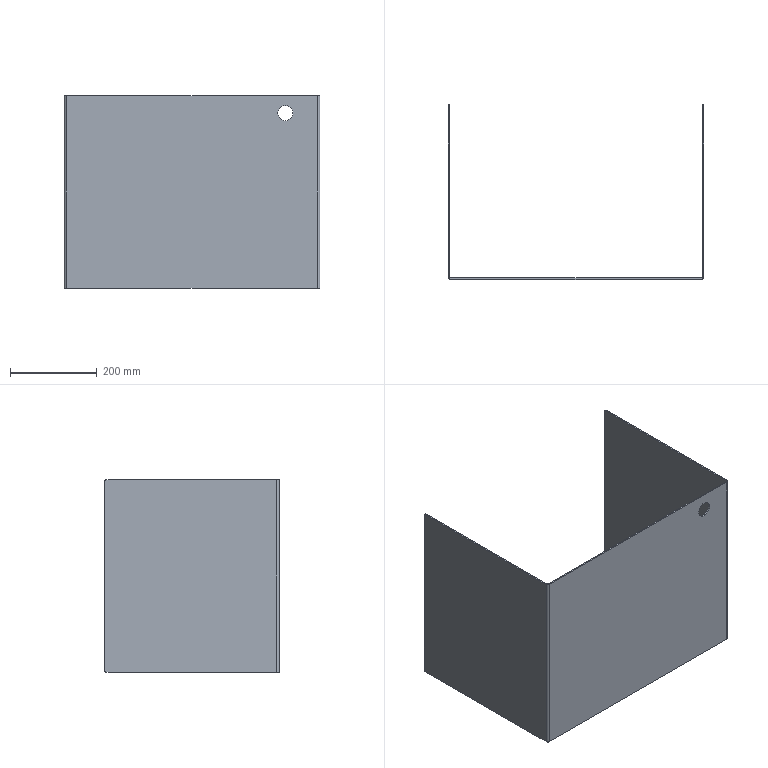Part | SolidWorks | features Fillet 1, FlatPattern 1, ICE 1, SMBaseFlange 1, SheetMetal 1 | 1 solid | 28 faces | box 590 x 403 x 444 mm | volume 1843422 mm3 | plane 18 | cylinder 10 | commonest cylinder face diameters 6.4 x4 6 x2 12 x2 35 x2
STEP:
#1=CARTESIAN_POINT('',(510.,0.,164.5));
#2=VERTEX_POINT('',#1);
#3=CARTESIAN_POINT('',(510.,0.,199.5));
#4=VERTEX_POINT('',#3);
#5=CARTESIAN_POINT('',(510.,0.,182.));
#6=DIRECTION('',(0.,1.,0.));
#7=DIRECTION('',(0.,0.,1.));
#8=AXIS2_PLACEMENT_3D('',#5,#6,#7);
#9=CIRCLE('',#8,17.5);
#10=EDGE_CURVE('',#2,#4,#9,.T.);
#11=ORIENTED_EDGE('',*,*,#10,.F.);
#12=CARTESIAN_POINT('',(510.,3.,164.5));
#13=VERTEX_POINT('',#12);
#14=CARTESIAN_POINT('',(510.,0.,164.5));
#15=DIRECTION('',(0.,1.,0.));
#16=VECTOR('',#15,1000.);
#17=LINE('',#14,#16);
#18=EDGE_CURVE('',#2,#13,#17,.T.);
#19=ORIENTED_EDGE('',*,*,#18,.T.);
#20=CARTESIAN_POINT('',(510.,3.,199.5));
#21=VERTEX_POINT('',#20);
#22=CARTESIAN_POINT('',(510.,3.,182.));
#23=DIRECTION('',(0.,1.,0.));
#24=DIRECTION('',(0.,0.,1.));
#25=AXIS2_PLACEMENT_3D('',#22,#23,#24);
#26=CIRCLE('',#25,17.5);
#27=EDGE_CURVE('',#13,#21,#26,.T.);
#28=ORIENTED_EDGE('',*,*,#27,.T.);
#29=CARTESIAN_POINT('',(510.,0.,199.5));
#30=DIRECTION('',(0.,1.,0.));
#31=VECTOR('',#30,1000.);
#32=LINE('',#29,#31);
#33=EDGE_CURVE('',#4,#21,#32,.T.);
#34=ORIENTED_EDGE('',*,*,#33,.F.);
#35=EDGE_LOOP('',(#11,#19,#28,#34));
#36=FACE_OUTER_BOUND('',#35,.T.);
#37=CARTESIAN_POINT('',(510.,0.,182.));
#38=DIRECTION('',(0.,1.,0.));
#39=DIRECTION('',(0.,0.,1.));
#40=AXIS2_PLACEMENT_3D('',#37,#38,#39);
#41=CYLINDRICAL_SURFACE('',#40,17.5);
#42=ADVANCED_FACE('',(#36),#41,.F.);
#43=CARTESIAN_POINT('',(0.,6.,222.));
#44=VERTEX_POINT('',#43);
#45=CARTESIAN_POINT('',(3.,6.,222.));
#46=VERTEX_POINT('',#45);
#47=CARTESIAN_POINT('',(0.,6.,222.));
#48=DIRECTION('',(1.,0.,0.));
#49=VECTOR('',#48,1000.);
#50=LINE('',#47,#49);
#51=EDGE_CURVE('',#44,#46,#50,.T.);
#52=ORIENTED_EDGE('',*,*,#51,.F.);
#53=CARTESIAN_POINT('',(6.,0.,222.));
#54=VERTEX_POINT('',#53);
#55=CARTESIAN_POINT('',(6.,6.,222.));
#56=DIRECTION('',(0.,0.,1.));
#57=DIRECTION('',(-1.,0.,0.));
#58=AXIS2_PLACEMENT_3D('',#55,#56,#57);
#59=CIRCLE('',#58,6.);
#60=EDGE_CURVE('',#44,#54,#59,.T.);
#61=ORIENTED_EDGE('',*,*,#60,.T.);
#62=CARTESIAN_POINT('',(6.,3.,222.));
#63=VERTEX_POINT('',#62);
#64=CARTESIAN_POINT('',(6.,3.,222.));
#65=DIRECTION('',(0.,-1.,0.));
#66=VECTOR('',#65,1000.);
#67=LINE('',#64,#66);
#68=EDGE_CURVE('',#63,#54,#67,.T.);
#69=ORIENTED_EDGE('',*,*,#68,.F.);
#70=CARTESIAN_POINT('',(6.,6.,222.));
#71=DIRECTION('',(0.,0.,1.));
#72=DIRECTION('',(1.,0.,0.));
#73=AXIS2_PLACEMENT_3D('',#70,#71,#72);
#74=CIRCLE('',#73,3.);
#75=EDGE_CURVE('',#46,#63,#74,.T.);
#76=ORIENTED_EDGE('',*,*,#75,.F.);
#77=EDGE_LOOP('',(#52,#61,#69,#76));
#78=FACE_OUTER_BOUND('',#77,.T.);
#79=CARTESIAN_POINT('',(0.,6.,222.));
#80=DIRECTION('',(0.,0.,1.));
#81=DIRECTION('',(1.,0.,0.));
#82=AXIS2_PLACEMENT_3D('',#79,#80,#81);
#83=PLANE('',#82);
#84=ADVANCED_FACE('',(#78),#83,.T.);
#85=CARTESIAN_POINT('',(3.,399.8,222.));
#86=VERTEX_POINT('',#85);
#87=CARTESIAN_POINT('',(3.,0.,222.));
#88=DIRECTION('',(0.,-1.,0.));
#89=VECTOR('',#88,1000.);
#90=LINE('',#87,#89);
#91=EDGE_CURVE('',#86,#46,#90,.T.);
#92=ORIENTED_EDGE('',*,*,#91,.F.);
#93=CARTESIAN_POINT('',(0.,399.8,222.));
#94=VERTEX_POINT('',#93);
#95=CARTESIAN_POINT('',(6.,399.8,222.));
#96=DIRECTION('',(-1.,0.,0.));
#97=VECTOR('',#96,1000.);
#98=LINE('',#95,#97);
#99=EDGE_CURVE('',#86,#94,#98,.T.);
#100=ORIENTED_EDGE('',*,*,#99,.T.);
#101=CARTESIAN_POINT('',(0.,0.,222.));
#102=DIRECTION('',(0.,-1.,0.));
#103=VECTOR('',#102,1000.);
#104=LINE('',#101,#103);
#105=EDGE_CURVE('',#94,#44,#104,.T.);
#106=ORIENTED_EDGE('',*,*,#105,.T.);
#107=ORIENTED_EDGE('',*,*,#51,.T.);
#108=EDGE_LOOP('',(#92,#100,#106,#107));
#109=FACE_OUTER_BOUND('',#108,.T.);
#110=CARTESIAN_POINT('',(6.,3.,222.));
#111=DIRECTION('',(0.,0.,1.));
#112=DIRECTION('',(1.,0.,0.));
#113=AXIS2_PLACEMENT_3D('',#110,#111,#112);
#114=PLANE('',#113);
#115=ADVANCED_FACE('',(#109),#114,.T.);
#116=CARTESIAN_POINT('',(6.,0.,-222.));
#117=VERTEX_POINT('',#116);
#118=CARTESIAN_POINT('',(6.,3.,-222.));
#119=VERTEX_POINT('',#118);
#120=CARTESIAN_POINT('',(6.,0.,-222.));
#121=DIRECTION('',(0.,1.,0.));
#122=VECTOR('',#121,1000.);
#123=LINE('',#120,#122);
#124=EDGE_CURVE('',#117,#119,#123,.T.);
#125=ORIENTED_EDGE('',*,*,#124,.F.);
#126=CARTESIAN_POINT('',(0.,6.,-222.));
#127=VERTEX_POINT('',#126);
#128=CARTESIAN_POINT('',(6.,6.,-222.));
#129=DIRECTION('',(0.,0.,1.));
#130=DIRECTION('',(-1.,0.,0.));
#131=AXIS2_PLACEMENT_3D('',#128,#129,#130);
#132=CIRCLE('',#131,6.);
#133=EDGE_CURVE('',#127,#117,#132,.T.);
#134=ORIENTED_EDGE('',*,*,#133,.F.);
#135=CARTESIAN_POINT('',(3.,6.,-222.));
#136=VERTEX_POINT('',#135);
#137=CARTESIAN_POINT('',(3.,6.,-222.));
#138=DIRECTION('',(-1.,0.,0.));
#139=VECTOR('',#138,1000.);
#140=LINE('',#137,#139);
#141=EDGE_CURVE('',#136,#127,#140,.T.);
#142=ORIENTED_EDGE('',*,*,#141,.F.);
#143=CARTESIAN_POINT('',(6.,6.,-222.));
#144=DIRECTION('',(0.,0.,1.));
#145=DIRECTION('',(1.,0.,0.));
#146=AXIS2_PLACEMENT_3D('',#143,#144,#145);
#147=CIRCLE('',#146,3.);
#148=EDGE_CURVE('',#136,#119,#147,.T.);
#149=ORIENTED_EDGE('',*,*,#148,.T.);
#150=EDGE_LOOP('',(#125,#134,#142,#149));
#151=FACE_OUTER_BOUND('',#150,.T.);
#152=CARTESIAN_POINT('',(6.,0.,-222.));
#153=DIRECTION('',(0.,0.,-1.));
#154=DIRECTION('',(-1.,0.,0.));
#155=AXIS2_PLACEMENT_3D('',#152,#153,#154);
#156=PLANE('',#155);
#157=ADVANCED_FACE('',(#151),#156,.T.);
#158=CARTESIAN_POINT('',(584.,0.,-222.));
#159=VERTEX_POINT('',#158);
#160=CARTESIAN_POINT('',(0.,0.,-222.));
#161=DIRECTION('',(1.,0.,0.));
#162=VECTOR('',#161,1000.);
#163=LINE('',#160,#162);
#164=EDGE_CURVE('',#117,#159,#163,.T.);
#165=ORIENTED_EDGE('',*,*,#164,.F.);
#166=ORIENTED_EDGE('',*,*,#124,.T.);
#167=CARTESIAN_POINT('',(584.,3.,-222.));
#168=VERTEX_POINT('',#167);
#169=CARTESIAN_POINT('',(0.,3.,-222.));
#170=DIRECTION('',(1.,0.,0.));
#171=VECTOR('',#170,1000.);
#172=LINE('',#169,#171);
#173=EDGE_CURVE('',#119,#168,#172,.T.);
#174=ORIENTED_EDGE('',*,*,#173,.T.);
#175=CARTESIAN_POINT('',(584.,3.,-222.));
#176=DIRECTION('',(0.,-1.,0.));
#177=VECTOR('',#176,1000.);
#178=LINE('',#175,#177);
#179=EDGE_CURVE('',#168,#159,#178,.T.);
#180=ORIENTED_EDGE('',*,*,#179,.T.);
#181=EDGE_LOOP('',(#165,#166,#174,#180));
#182=FACE_OUTER_BOUND('',#181,.T.);
#183=CARTESIAN_POINT('',(3.,6.,-222.));
#184=DIRECTION('',(0.,0.,-1.));
#185=DIRECTION('',(-1.,0.,0.));
#186=AXIS2_PLACEMENT_3D('',#183,#184,#185);
#187=PLANE('',#186);
#188=ADVANCED_FACE('',(#182),#187,.T.);
#189=CARTESIAN_POINT('',(584.,0.,222.));
#190=VERTEX_POINT('',#189);
#191=CARTESIAN_POINT('',(584.,3.,222.));
#192=VERTEX_POINT('',#191);
#193=CARTESIAN_POINT('',(584.,0.,222.));
#194=DIRECTION('',(0.,1.,0.));
#195=VECTOR('',#194,1000.);
#196=LINE('',#193,#195);
#197=EDGE_CURVE('',#190,#192,#196,.T.);
#198=ORIENTED_EDGE('',*,*,#197,.F.);
#199=CARTESIAN_POINT('',(590.,6.,222.));
#200=VERTEX_POINT('',#199);
#201=CARTESIAN_POINT('',(584.,6.,222.));
#202=DIRECTION('',(0.,0.,1.));
#203=DIRECTION('',(-1.,0.,0.));
#204=AXIS2_PLACEMENT_3D('',#201,#202,#203);
#205=CIRCLE('',#204,6.);
#206=EDGE_CURVE('',#190,#200,#205,.T.);
#207=ORIENTED_EDGE('',*,*,#206,.T.);
#208=CARTESIAN_POINT('',(587.,6.,222.));
#209=VERTEX_POINT('',#208);
#210=CARTESIAN_POINT('',(587.,6.,222.));
#211=DIRECTION('',(1.,0.,0.));
#212=VECTOR('',#211,1000.);
#213=LINE('',#210,#212);
#214=EDGE_CURVE('',#209,#200,#213,.T.);
#215=ORIENTED_EDGE('',*,*,#214,.F.);
#216=CARTESIAN_POINT('',(584.,6.,222.));
#217=DIRECTION('',(0.,0.,1.));
#218=DIRECTION('',(1.,0.,0.));
#219=AXIS2_PLACEMENT_3D('',#216,#217,#218);
#220=CIRCLE('',#219,3.);
#221=EDGE_CURVE('',#192,#209,#220,.T.);
#222=ORIENTED_EDGE('',*,*,#221,.F.);
#223=EDGE_LOOP('',(#198,#207,#215,#222));
#224=FACE_OUTER_BOUND('',#223,.T.);
#225=CARTESIAN_POINT('',(584.,0.,222.));
#226=DIRECTION('',(0.,0.,1.));
#227=DIRECTION('',(1.,0.,0.));
#228=AXIS2_PLACEMENT_3D('',#225,#226,#227);
#229=PLANE('',#228);
#230=ADVANCED_FACE('',(#224),#229,.T.);
#231=CARTESIAN_POINT('',(0.,0.,222.));
#232=DIRECTION('',(1.,0.,0.));
#233=VECTOR('',#232,1000.);
#234=LINE('',#231,#233);
#235=EDGE_CURVE('',#54,#190,#234,.T.);
#236=ORIENTED_EDGE('',*,*,#235,.T.);
#237=ORIENTED_EDGE('',*,*,#197,.T.);
#238=CARTESIAN_POINT('',(0.,3.,222.));
#239=DIRECTION('',(1.,0.,0.));
#240=VECTOR('',#239,1000.);
#241=LINE('',#238,#240);
#242=EDGE_CURVE('',#63,#192,#241,.T.);
#243=ORIENTED_EDGE('',*,*,#242,.F.);
#244=ORIENTED_EDGE('',*,*,#68,.T.);
#245=EDGE_LOOP('',(#236,#237,#243,#244));
#246=FACE_OUTER_BOUND('',#245,.T.);
#247=CARTESIAN_POINT('',(587.,6.,222.));
#248=DIRECTION('',(0.,0.,1.));
#249=DIRECTION('',(1.,0.,0.));
#250=AXIS2_PLACEMENT_3D('',#247,#248,#249);
#251=PLANE('',#250);
#252=ADVANCED_FACE('',(#246),#251,.T.);
#253=CARTESIAN_POINT('',(590.,6.,-222.));
#254=VERTEX_POINT('',#253);
#255=CARTESIAN_POINT('',(587.,6.,-222.));
#256=VERTEX_POINT('',#255);
#257=CARTESIAN_POINT('',(590.,6.,-222.));
#258=DIRECTION('',(-1.,0.,0.));
#259=VECTOR('',#258,1000.);
#260=LINE('',#257,#259);
#261=EDGE_CURVE('',#254,#256,#260,.T.);
#262=ORIENTED_EDGE('',*,*,#261,.F.);
#263=CARTESIAN_POINT('',(584.,6.,-222.));
#264=DIRECTION('',(0.,0.,1.));
#265=DIRECTION('',(-1.,0.,0.));
#266=AXIS2_PLACEMENT_3D('',#263,#264,#265);
#267=CIRCLE('',#266,6.);
#268=EDGE_CURVE('',#159,#254,#267,.T.);
#269=ORIENTED_EDGE('',*,*,#268,.F.);
#270=ORIENTED_EDGE('',*,*,#179,.F.);
#271=CARTESIAN_POINT('',(584.,6.,-222.));
#272=DIRECTION('',(0.,0.,1.));
#273=DIRECTION('',(1.,0.,0.));
#274=AXIS2_PLACEMENT_3D('',#271,#272,#273);
#275=CIRCLE('',#274,3.);
#276=EDGE_CURVE('',#168,#256,#275,.T.);
#277=ORIENTED_EDGE('',*,*,#276,.T.);
#278=EDGE_LOOP('',(#262,#269,#270,#277));
#279=FACE_OUTER_BOUND('',#278,.T.);
#280=CARTESIAN_POINT('',(590.,6.,-222.));
#281=DIRECTION('',(0.,0.,-1.));
#282=DIRECTION('',(-1.,0.,0.));
#283=AXIS2_PLACEMENT_3D('',#280,#281,#282);
#284=PLANE('',#283);
#285=ADVANCED_FACE('',(#279),#284,.T.);
#286=CARTESIAN_POINT('',(587.,399.8,-222.));
#287=VERTEX_POINT('',#286);
#288=CARTESIAN_POINT('',(587.,0.,-222.));
#289=DIRECTION('',(0.,1.,0.));
#290=VECTOR('',#289,1000.);
#291=LINE('',#288,#290);
#292=EDGE_CURVE('',#256,#287,#291,.T.);
#293=ORIENTED_EDGE('',*,*,#292,.T.);
#294=CARTESIAN_POINT('',(590.,399.8,-222.));
#295=VERTEX_POINT('',#294);
#296=CARTESIAN_POINT('',(584.,399.8,-222.));
#297=DIRECTION('',(1.,0.,0.));
#298=VECTOR('',#297,1000.);
#299=LINE('',#296,#298);
#300=EDGE_CURVE('',#287,#295,#299,.T.);
#301=ORIENTED_EDGE('',*,*,#300,.T.);
#302=CARTESIAN_POINT('',(590.,0.,-222.));
#303=DIRECTION('',(0.,1.,0.));
#304=VECTOR('',#303,1000.);
#305=LINE('',#302,#304);
#306=EDGE_CURVE('',#254,#295,#305,.T.);
#307=ORIENTED_EDGE('',*,*,#306,.F.);
#308=ORIENTED_EDGE('',*,*,#261,.T.);
#309=EDGE_LOOP('',(#293,#301,#307,#308));
#310=FACE_OUTER_BOUND('',#309,.T.);
#311=CARTESIAN_POINT('',(584.,3.,-222.));
#312=DIRECTION('',(0.,0.,-1.));
#313=DIRECTION('',(-1.,0.,0.));
#314=AXIS2_PLACEMENT_3D('',#311,#312,#313);
#315=PLANE('',#314);
#316=ADVANCED_FACE('',(#310),#315,.T.);
#317=ORIENTED_EDGE('',*,*,#306,.T.);
#318=CARTESIAN_POINT('',(590.,403.,-218.8));
#319=VERTEX_POINT('',#318);
#320=CARTESIAN_POINT('',(590.,399.8,-218.8));
#321=DIRECTION('',(1.,0.,0.));
#322=DIRECTION('',(0.,0.,1.));
#323=AXIS2_PLACEMENT_3D('',#320,#321,#322);
#324=CIRCLE('',#323,3.2);
#325=EDGE_CURVE('',#295,#319,#324,.T.);
#326=ORIENTED_EDGE('',*,*,#325,.T.);
#327=CARTESIAN_POINT('',(590.,403.,218.8));
#328=VERTEX_POINT('',#327);
#329=CARTESIAN_POINT('',(590.,403.,222.));
#330=DIRECTION('',(0.,0.,-1.));
#331=VECTOR('',#330,1000.);
#332=LINE('',#329,#331);
#333=EDGE_CURVE('',#328,#319,#332,.T.);
#334=ORIENTED_EDGE('',*,*,#333,.F.);
#335=CARTESIAN_POINT('',(590.,399.8,222.));
#336=VERTEX_POINT('',#335);
#337=CARTESIAN_POINT('',(590.,399.8,218.8));
#338=DIRECTION('',(1.,0.,0.));
#339=DIRECTION('',(0.,0.,1.));
#340=AXIS2_PLACEMENT_3D('',#337,#338,#339);
#341=CIRCLE('',#340,3.2);
#342=EDGE_CURVE('',#328,#336,#341,.T.);
#343=ORIENTED_EDGE('',*,*,#342,.T.);
#344=CARTESIAN_POINT('',(590.,0.,222.));
#345=DIRECTION('',(0.,1.,0.));
#346=VECTOR('',#345,1000.);
#347=LINE('',#344,#346);
#348=EDGE_CURVE('',#200,#336,#347,.T.);
#349=ORIENTED_EDGE('',*,*,#348,.F.);
#350=CARTESIAN_POINT('',(590.,6.,222.));
#351=DIRECTION('',(0.,0.,-1.));
#352=VECTOR('',#351,1000.);
#353=LINE('',#350,#352);
#354=EDGE_CURVE('',#200,#254,#353,.T.);
#355=ORIENTED_EDGE('',*,*,#354,.T.);
#356=EDGE_LOOP('',(#317,#326,#334,#343,#349,#355));
#357=FACE_OUTER_BOUND('',#356,.T.);
#358=CARTESIAN_POINT('',(590.,0.,222.));
#359=DIRECTION('',(-1.,0.,0.));
#360=DIRECTION('',(0.,0.,1.));
#361=AXIS2_PLACEMENT_3D('',#358,#359,#360);
#362=PLANE('',#361);
#363=ADVANCED_FACE('',(#357),#362,.F.);
#364=ORIENTED_EDGE('',*,*,#333,.T.);
#365=CARTESIAN_POINT('',(587.,403.,-218.8));
#366=VERTEX_POINT('',#365);
#367=CARTESIAN_POINT('',(587.,403.,-218.8));
#368=DIRECTION('',(-1.,0.,0.));
#369=VECTOR('',#368,1000.);
#370=LINE('',#367,#369);
#371=EDGE_CURVE('',#319,#366,#370,.T.);
#372=ORIENTED_EDGE('',*,*,#371,.T.);
#373=CARTESIAN_POINT('',(587.,403.,218.8));
#374=VERTEX_POINT('',#373);
#375=CARTESIAN_POINT('',(587.,403.,222.));
#376=DIRECTION('',(0.,0.,-1.));
#377=VECTOR('',#376,1000.);
#378=LINE('',#375,#377);
#379=EDGE_CURVE('',#374,#366,#378,.T.);
#380=ORIENTED_EDGE('',*,*,#379,.F.);
#381=CARTESIAN_POINT('',(587.,403.,218.8));
#382=DIRECTION('',(1.,0.,0.));
#383=VECTOR('',#382,1000.);
#384=LINE('',#381,#383);
#385=EDGE_CURVE('',#374,#328,#384,.T.);
#386=ORIENTED_EDGE('',*,*,#385,.T.);
#387=EDGE_LOOP('',(#364,#372,#380,#386));
#388=FACE_OUTER_BOUND('',#387,.T.);
#389=CARTESIAN_POINT('',(587.,403.,222.));
#390=DIRECTION('',(0.,1.,0.));
#391=DIRECTION('',(0.,0.,1.));
#392=AXIS2_PLACEMENT_3D('',#389,#390,#391);
#393=PLANE('',#392);
#394=ADVANCED_FACE('',(#388),#393,.T.);
#395=ORIENTED_EDGE('',*,*,#379,.T.);
#396=CARTESIAN_POINT('',(587.,399.8,-218.8));
#397=DIRECTION('',(-1.,0.,0.));
#398=DIRECTION('',(0.,0.,1.));
#399=AXIS2_PLACEMENT_3D('',#396,#397,#398);
#400=CIRCLE('',#399,3.2);
#401=EDGE_CURVE('',#366,#287,#400,.T.);
#402=ORIENTED_EDGE('',*,*,#401,.T.);
#403=ORIENTED_EDGE('',*,*,#292,.F.);
#404=CARTESIAN_POINT('',(587.,6.,222.));
#405=DIRECTION('',(0.,0.,-1.));
#406=VECTOR('',#405,1000.);
#407=LINE('',#404,#406);
#408=EDGE_CURVE('',#209,#256,#407,.T.);
#409=ORIENTED_EDGE('',*,*,#408,.F.);
#410=CARTESIAN_POINT('',(587.,399.8,222.));
#411=VERTEX_POINT('',#410);
#412=CARTESIAN_POINT('',(587.,0.,222.));
#413=DIRECTION('',(0.,1.,0.));
#414=VECTOR('',#413,1000.);
#415=LINE('',#412,#414);
#416=EDGE_CURVE('',#209,#411,#415,.T.);
#417=ORIENTED_EDGE('',*,*,#416,.T.);
#418=CARTESIAN_POINT('',(587.,399.8,218.8));
#419=DIRECTION('',(-1.,0.,0.));
#420=DIRECTION('',(0.,0.,1.));
#421=AXIS2_PLACEMENT_3D('',#418,#419,#420);
#422=CIRCLE('',#421,3.2);
#423=EDGE_CURVE('',#411,#374,#422,.T.);
#424=ORIENTED_EDGE('',*,*,#423,.T.);
#425=EDGE_LOOP('',(#395,#402,#403,#409,#417,#424));
#426=FACE_OUTER_BOUND('',#425,.T.);
#427=CARTESIAN_POINT('',(587.,0.,222.));
#428=DIRECTION('',(-1.,0.,0.));
#429=DIRECTION('',(0.,0.,1.));
#430=AXIS2_PLACEMENT_3D('',#427,#428,#429);
#431=PLANE('',#430);
#432=ADVANCED_FACE('',(#426),#431,.T.);
#433=ORIENTED_EDGE('',*,*,#276,.F.);
#434=CARTESIAN_POINT('',(584.,3.,222.));
#435=DIRECTION('',(0.,0.,-1.));
#436=VECTOR('',#435,1000.);
#437=LINE('',#434,#436);
#438=EDGE_CURVE('',#192,#168,#437,.T.);
#439=ORIENTED_EDGE('',*,*,#438,.F.);
#440=ORIENTED_EDGE('',*,*,#221,.T.);
#441=ORIENTED_EDGE('',*,*,#408,.T.);
#442=EDGE_LOOP('',(#433,#439,#440,#441));
#443=FACE_OUTER_BOUND('',#442,.T.);
#444=CARTESIAN_POINT('',(584.,6.,222.));
#445=DIRECTION('',(0.,0.,-1.));
#446=DIRECTION('',(-1.,0.,0.));
#447=AXIS2_PLACEMENT_3D('',#444,#445,#446);
#448=CYLINDRICAL_SURFACE('',#447,3.);
#449=ADVANCED_FACE('',(#443),#448,.F.);
#450=CARTESIAN_POINT('',(510.,3.,182.));
#451=DIRECTION('',(0.,1.,0.));
#452=DIRECTION('',(0.,0.,1.));
#453=AXIS2_PLACEMENT_3D('',#450,#451,#452);
#454=CIRCLE('',#453,17.5);
#455=EDGE_CURVE('',#21,#13,#454,.T.);
#456=ORIENTED_EDGE('',*,*,#455,.F.);
#457=ORIENTED_EDGE('',*,*,#27,.F.);
#458=EDGE_LOOP('',(#456,#457));
#459=FACE_BOUND('',#458,.T.);
#460=ORIENTED_EDGE('',*,*,#173,.F.);
#461=CARTESIAN_POINT('',(6.,3.,222.));
#462=DIRECTION('',(0.,0.,-1.));
#463=VECTOR('',#462,1000.);
#464=LINE('',#461,#463);
#465=EDGE_CURVE('',#63,#119,#464,.T.);
#466=ORIENTED_EDGE('',*,*,#465,.F.);
#467=ORIENTED_EDGE('',*,*,#242,.T.);
#468=ORIENTED_EDGE('',*,*,#438,.T.);
#469=EDGE_LOOP('',(#460,#466,#467,#468));
#470=FACE_OUTER_BOUND('',#469,.T.);
#471=CARTESIAN_POINT('',(0.,3.,222.));
#472=DIRECTION('',(0.,1.,0.));
#473=DIRECTION('',(0.,0.,1.));
#474=AXIS2_PLACEMENT_3D('',#471,#472,#473);
#475=PLANE('',#474);
#476=ADVANCED_FACE('',(#459,#470),#475,.T.);
#477=ORIENTED_EDGE('',*,*,#148,.F.);
#478=CARTESIAN_POINT('',(3.,6.,222.));
#479=DIRECTION('',(0.,0.,-1.));
#480=VECTOR('',#479,1000.);
#481=LINE('',#478,#480);
#482=EDGE_CURVE('',#46,#136,#481,.T.);
#483=ORIENTED_EDGE('',*,*,#482,.F.);
#484=ORIENTED_EDGE('',*,*,#75,.T.);
#485=ORIENTED_EDGE('',*,*,#465,.T.);
#486=EDGE_LOOP('',(#477,#483,#484,#485));
#487=FACE_OUTER_BOUND('',#486,.T.);
#488=CARTESIAN_POINT('',(6.,6.,222.));
#489=DIRECTION('',(0.,0.,-1.));
#490=DIRECTION('',(-1.,0.,0.));
#491=AXIS2_PLACEMENT_3D('',#488,#489,#490);
#492=CYLINDRICAL_SURFACE('',#491,3.);
#493=ADVANCED_FACE('',(#487),#492,.F.);
#494=CARTESIAN_POINT('',(3.,403.,218.8));
#495=VERTEX_POINT('',#494);
#496=CARTESIAN_POINT('',(3.,403.,-218.8));
#497=VERTEX_POINT('',#496);
#498=CARTESIAN_POINT('',(3.,403.,222.));
#499=DIRECTION('',(0.,0.,-1.));
#500=VECTOR('',#499,1000.);
#501=LINE('',#498,#500);
#502=EDGE_CURVE('',#495,#497,#501,.T.);
#503=ORIENTED_EDGE('',*,*,#502,.F.);
#504=CARTESIAN_POINT('',(3.,399.8,218.8));
#505=DIRECTION('',(1.,0.,0.));
#506=DIRECTION('',(0.,0.,-1.));
#507=AXIS2_PLACEMENT_3D('',#504,#505,#506);
#508=CIRCLE('',#507,3.2);
#509=EDGE_CURVE('',#495,#86,#508,.T.);
#510=ORIENTED_EDGE('',*,*,#509,.T.);
#511=ORIENTED_EDGE('',*,*,#91,.T.);
#512=ORIENTED_EDGE('',*,*,#482,.T.);
#513=CARTESIAN_POINT('',(3.,399.8,-222.));
#514=VERTEX_POINT('',#513);
#515=CARTESIAN_POINT('',(3.,0.,-222.));
#516=DIRECTION('',(0.,-1.,0.));
#517=VECTOR('',#516,1000.);
#518=LINE('',#515,#517);
#519=EDGE_CURVE('',#514,#136,#518,.T.);
#520=ORIENTED_EDGE('',*,*,#519,.F.);
#521=CARTESIAN_POINT('',(3.,399.8,-218.8));
#522=DIRECTION('',(1.,0.,0.));
#523=DIRECTION('',(0.,0.,-1.));
#524=AXIS2_PLACEMENT_3D('',#521,#522,#523);
#525=CIRCLE('',#524,3.2);
#526=EDGE_CURVE('',#514,#497,#525,.T.);
#527=ORIENTED_EDGE('',*,*,#526,.T.);
#528=EDGE_LOOP('',(#503,#510,#511,#512,#520,#527));
#529=FACE_OUTER_BOUND('',#528,.T.);
#530=CARTESIAN_POINT('',(3.,0.,222.));
#531=DIRECTION('',(1.,0.,0.));
#532=DIRECTION('',(0.,0.,-1.));
#533=AXIS2_PLACEMENT_3D('',#530,#531,#532);
#534=PLANE('',#533);
#535=ADVANCED_FACE('',(#529),#534,.T.);
#536=CARTESIAN_POINT('',(0.,403.,218.8));
#537=VERTEX_POINT('',#536);
#538=CARTESIAN_POINT('',(0.,403.,-218.8));
#539=VERTEX_POINT('',#538);
#540=CARTESIAN_POINT('',(0.,403.,222.));
#541=DIRECTION('',(0.,0.,-1.));
#542=VECTOR('',#541,1000.);
#543=LINE('',#540,#542);
#544=EDGE_CURVE('',#537,#539,#543,.T.);
#545=ORIENTED_EDGE('',*,*,#544,.F.);
#546=CARTESIAN_POINT('',(0.,403.,218.8));
#547=DIRECTION('',(1.,0.,0.));
#548=VECTOR('',#547,1000.);
#549=LINE('',#546,#548);
#550=EDGE_CURVE('',#537,#495,#549,.T.);
#551=ORIENTED_EDGE('',*,*,#550,.T.);
#552=ORIENTED_EDGE('',*,*,#502,.T.);
#553=CARTESIAN_POINT('',(0.,403.,-218.8));
#554=DIRECTION('',(-1.,0.,0.));
#555=VECTOR('',#554,1000.);
#556=LINE('',#553,#555);
#557=EDGE_CURVE('',#497,#539,#556,.T.);
#558=ORIENTED_EDGE('',*,*,#557,.T.);
#559=EDGE_LOOP('',(#545,#551,#552,#558));
#560=FACE_OUTER_BOUND('',#559,.T.);
#561=CARTESIAN_POINT('',(0.,403.,222.));
#562=DIRECTION('',(0.,1.,0.));
#563=DIRECTION('',(0.,0.,1.));
#564=AXIS2_PLACEMENT_3D('',#561,#562,#563);
#565=PLANE('',#564);
#566=ADVANCED_FACE('',(#560),#565,.T.);
#567=ORIENTED_EDGE('',*,*,#105,.F.);
#568=CARTESIAN_POINT('',(0.,399.8,218.8));
#569=DIRECTION('',(-1.,0.,0.));
#570=DIRECTION('',(0.,0.,-1.));
#571=AXIS2_PLACEMENT_3D('',#568,#569,#570);
#572=CIRCLE('',#571,3.2);
#573=EDGE_CURVE('',#94,#537,#572,.T.);
#574=ORIENTED_EDGE('',*,*,#573,.T.);
#575=ORIENTED_EDGE('',*,*,#544,.T.);
#576=CARTESIAN_POINT('',(0.,399.8,-222.));
#577=VERTEX_POINT('',#576);
#578=CARTESIAN_POINT('',(0.,399.8,-218.8));
#579=DIRECTION('',(-1.,0.,0.));
#580=DIRECTION('',(0.,0.,-1.));
#581=AXIS2_PLACEMENT_3D('',#578,#579,#580);
#582=CIRCLE('',#581,3.2);
#583=EDGE_CURVE('',#539,#577,#582,.T.);
#584=ORIENTED_EDGE('',*,*,#583,.T.);
#585=CARTESIAN_POINT('',(0.,0.,-222.));
#586=DIRECTION('',(0.,-1.,0.));
#587=VECTOR('',#586,1000.);
#588=LINE('',#585,#587);
#589=EDGE_CURVE('',#577,#127,#588,.T.);
#590=ORIENTED_EDGE('',*,*,#589,.T.);
#591=CARTESIAN_POINT('',(0.,6.,222.));
#592=DIRECTION('',(0.,0.,-1.));
#593=VECTOR('',#592,1000.);
#594=LINE('',#591,#593);
#595=EDGE_CURVE('',#44,#127,#594,.T.);
#596=ORIENTED_EDGE('',*,*,#595,.F.);
#597=EDGE_LOOP('',(#567,#574,#575,#584,#590,#596));
#598=FACE_OUTER_BOUND('',#597,.T.);
#599=CARTESIAN_POINT('',(0.,0.,222.));
#600=DIRECTION('',(1.,0.,0.));
#601=DIRECTION('',(0.,0.,-1.));
#602=AXIS2_PLACEMENT_3D('',#599,#600,#601);
#603=PLANE('',#602);
#604=ADVANCED_FACE('',(#598),#603,.F.);
#605=ORIENTED_EDGE('',*,*,#133,.T.);
#606=CARTESIAN_POINT('',(6.,0.,222.));
#607=DIRECTION('',(0.,0.,-1.));
#608=VECTOR('',#607,1000.);
#609=LINE('',#606,#608);
#610=EDGE_CURVE('',#54,#117,#609,.T.);
#611=ORIENTED_EDGE('',*,*,#610,.F.);
#612=ORIENTED_EDGE('',*,*,#60,.F.);
#613=ORIENTED_EDGE('',*,*,#595,.T.);
#614=EDGE_LOOP('',(#605,#611,#612,#613));
#615=FACE_OUTER_BOUND('',#614,.T.);
#616=CARTESIAN_POINT('',(6.,6.,222.));
#617=DIRECTION('',(0.,0.,-1.));
#618=DIRECTION('',(-1.,0.,0.));
#619=AXIS2_PLACEMENT_3D('',#616,#617,#618);
#620=CYLINDRICAL_SURFACE('',#619,6.);
#621=ADVANCED_FACE('',(#615),#620,.T.);
#622=CARTESIAN_POINT('',(510.,0.,182.));
#623=DIRECTION('',(0.,1.,0.));
#624=DIRECTION('',(0.,0.,1.));
#625=AXIS2_PLACEMENT_3D('',#622,#623,#624);
#626=CIRCLE('',#625,17.5);
#627=EDGE_CURVE('',#4,#2,#626,.T.);
#628=ORIENTED_EDGE('',*,*,#627,.T.);
#629=ORIENTED_EDGE('',*,*,#10,.T.);
#630=EDGE_LOOP('',(#628,#629));
#631=FACE_BOUND('',#630,.T.);
#632=ORIENTED_EDGE('',*,*,#164,.T.);
#633=CARTESIAN_POINT('',(584.,0.,222.));
#634=DIRECTION('',(0.,0.,-1.));
#635=VECTOR('',#634,1000.);
#636=LINE('',#633,#635);
#637=EDGE_CURVE('',#190,#159,#636,.T.);
#638=ORIENTED_EDGE('',*,*,#637,.F.);
#639=ORIENTED_EDGE('',*,*,#235,.F.);
#640=ORIENTED_EDGE('',*,*,#610,.T.);
#641=EDGE_LOOP('',(#632,#638,#639,#640));
#642=FACE_OUTER_BOUND('',#641,.T.);
#643=CARTESIAN_POINT('',(0.,0.,222.));
#644=DIRECTION('',(0.,1.,0.));
#645=DIRECTION('',(0.,0.,1.));
#646=AXIS2_PLACEMENT_3D('',#643,#644,#645);
#647=PLANE('',#646);
#648=ADVANCED_FACE('',(#631,#642),#647,.F.);
#649=ORIENTED_EDGE('',*,*,#268,.T.);
#650=ORIENTED_EDGE('',*,*,#354,.F.);
#651=ORIENTED_EDGE('',*,*,#206,.F.);
#652=ORIENTED_EDGE('',*,*,#637,.T.);
#653=EDGE_LOOP('',(#649,#650,#651,#652));
#654=FACE_OUTER_BOUND('',#653,.T.);
#655=CARTESIAN_POINT('',(584.,6.,222.));
#656=DIRECTION('',(0.,0.,-1.));
#657=DIRECTION('',(-1.,0.,0.));
#658=AXIS2_PLACEMENT_3D('',#655,#656,#657);
#659=CYLINDRICAL_SURFACE('',#658,6.);
#660=ADVANCED_FACE('',(#654),#659,.T.);
#661=ORIENTED_EDGE('',*,*,#348,.T.);
#662=CARTESIAN_POINT('',(584.,399.8,222.));
#663=DIRECTION('',(-1.,0.,0.));
#664=VECTOR('',#663,1000.);
#665=LINE('',#662,#664);
#666=EDGE_CURVE('',#336,#411,#665,.T.);
#667=ORIENTED_EDGE('',*,*,#666,.T.);
#668=ORIENTED_EDGE('',*,*,#416,.F.);
#669=ORIENTED_EDGE('',*,*,#214,.T.);
#670=EDGE_LOOP('',(#661,#667,#668,#669));
#671=FACE_OUTER_BOUND('',#670,.T.);
#672=CARTESIAN_POINT('',(584.,6.,222.));
#673=DIRECTION('',(0.,0.,1.));
#674=DIRECTION('',(1.,0.,0.));
#675=AXIS2_PLACEMENT_3D('',#672,#673,#674);
#676=PLANE('',#675);
#677=ADVANCED_FACE('',(#671),#676,.T.);
#678=ORIENTED_EDGE('',*,*,#589,.F.);
#679=CARTESIAN_POINT('',(3.,399.8,-222.));
#680=DIRECTION('',(1.,0.,0.));
#681=VECTOR('',#680,1000.);
#682=LINE('',#679,#681);
#683=EDGE_CURVE('',#577,#514,#682,.T.);
#684=ORIENTED_EDGE('',*,*,#683,.T.);
#685=ORIENTED_EDGE('',*,*,#519,.T.);
#686=ORIENTED_EDGE('',*,*,#141,.T.);
#687=EDGE_LOOP('',(#678,#684,#685,#686));
#688=FACE_OUTER_BOUND('',#687,.T.);
#689=CARTESIAN_POINT('',(584.,6.,-222.));
#690=DIRECTION('',(0.,0.,1.));
#691=DIRECTION('',(1.,0.,0.));
#692=AXIS2_PLACEMENT_3D('',#689,#690,#691);
#693=PLANE('',#692);
#694=ADVANCED_FACE('',(#688),#693,.F.);
#695=ORIENTED_EDGE('',*,*,#18,.F.);
#696=ORIENTED_EDGE('',*,*,#627,.F.);
#697=ORIENTED_EDGE('',*,*,#33,.T.);
#698=ORIENTED_EDGE('',*,*,#455,.T.);
#699=EDGE_LOOP('',(#695,#696,#697,#698));
#700=FACE_OUTER_BOUND('',#699,.T.);
#701=CARTESIAN_POINT('',(510.,0.,182.));
#702=DIRECTION('',(0.,1.,0.));
#703=DIRECTION('',(0.,0.,1.));
#704=AXIS2_PLACEMENT_3D('',#701,#702,#703);
#705=CYLINDRICAL_SURFACE('',#704,17.5);
#706=ADVANCED_FACE('',(#700),#705,.F.);
#707=ORIENTED_EDGE('',*,*,#401,.F.);
#708=ORIENTED_EDGE('',*,*,#371,.F.);
#709=ORIENTED_EDGE('',*,*,#325,.F.);
#710=ORIENTED_EDGE('',*,*,#300,.F.);
#711=EDGE_LOOP('',(#707,#708,#709,#710));
#712=FACE_OUTER_BOUND('',#711,.T.);
#713=CARTESIAN_POINT('',(584.,399.8,-218.8));
#714=DIRECTION('',(1.,0.,0.));
#715=DIRECTION('',(0.,0.,-1.));
#716=AXIS2_PLACEMENT_3D('',#713,#714,#715);
#717=CYLINDRICAL_SURFACE('',#716,3.2);
#718=ADVANCED_FACE('',(#712),#717,.T.);
#719=ORIENTED_EDGE('',*,*,#423,.F.);
#720=ORIENTED_EDGE('',*,*,#666,.F.);
#721=ORIENTED_EDGE('',*,*,#342,.F.);
#722=ORIENTED_EDGE('',*,*,#385,.F.);
#723=EDGE_LOOP('',(#719,#720,#721,#722));
#724=FACE_OUTER_BOUND('',#723,.T.);
#725=CARTESIAN_POINT('',(587.,399.8,218.8));
#726=DIRECTION('',(1.,0.,0.));
#727=DIRECTION('',(0.,0.,-1.));
#728=AXIS2_PLACEMENT_3D('',#725,#726,#727);
#729=CYLINDRICAL_SURFACE('',#728,3.2);
#730=ADVANCED_FACE('',(#724),#729,.T.);
#731=ORIENTED_EDGE('',*,*,#573,.F.);
#732=ORIENTED_EDGE('',*,*,#99,.F.);
#733=ORIENTED_EDGE('',*,*,#509,.F.);
#734=ORIENTED_EDGE('',*,*,#550,.F.);
#735=EDGE_LOOP('',(#731,#732,#733,#734));
#736=FACE_OUTER_BOUND('',#735,.T.);
#737=CARTESIAN_POINT('',(0.,399.8,218.8));
#738=DIRECTION('',(1.,0.,0.));
#739=DIRECTION('',(0.,0.,-1.));
#740=AXIS2_PLACEMENT_3D('',#737,#738,#739);
#741=CYLINDRICAL_SURFACE('',#740,3.2);
#742=ADVANCED_FACE('',(#736),#741,.T.);
#743=ORIENTED_EDGE('',*,*,#583,.F.);
#744=ORIENTED_EDGE('',*,*,#557,.F.);
#745=ORIENTED_EDGE('',*,*,#526,.F.);
#746=ORIENTED_EDGE('',*,*,#683,.F.);
#747=EDGE_LOOP('',(#743,#744,#745,#746));
#748=FACE_OUTER_BOUND('',#747,.T.);
#749=CARTESIAN_POINT('',(584.,399.8,-218.8));
#750=DIRECTION('',(-1.,0.,0.));
#751=DIRECTION('',(0.,0.,1.));
#752=AXIS2_PLACEMENT_3D('',#749,#750,#751);
#753=CYLINDRICAL_SURFACE('',#752,3.2);
#754=ADVANCED_FACE('',(#748),#753,.T.);
#755=CLOSED_SHELL('',(#42,#84,#115,#157,#188,#230,#252,#285,#316,#363,#394,#432,#449,#476,#493,#535,#566,#604,#621,#648,#660,#677,#694,#706,#718,#730,#742,#754));
#756=MANIFOLD_SOLID_BREP('',#755);
#757=CARTESIAN_POINT('',(0.,0.,0.));
#758=DIRECTION('',(0.,0.,1.));
#759=DIRECTION('',(1.,0.,0.));
#760=AXIS2_PLACEMENT_3D('',#757,#758,#759);
#761=(LENGTH_UNIT()NAMED_UNIT(*)SI_UNIT(.MILLI.,.METRE.));
#762=UNCERTAINTY_MEASURE_WITH_UNIT(LENGTH_MEASURE(0.00001),#761,'','');
#763=(NAMED_UNIT(*)PLANE_ANGLE_UNIT()SI_UNIT($,.RADIAN.));
#764=(NAMED_UNIT(*)SI_UNIT($,.STERADIAN.)SOLID_ANGLE_UNIT());
#765=(GEOMETRIC_REPRESENTATION_CONTEXT(3)GLOBAL_UNCERTAINTY_ASSIGNED_CONTEXT((#762))GLOBAL_UNIT_ASSIGNED_CONTEXT((#761,#763,#764))REPRESENTATION_CONTEXT('',''));
#766=ADVANCED_BREP_SHAPE_REPRESENTATION('',(#756,#760),#765);